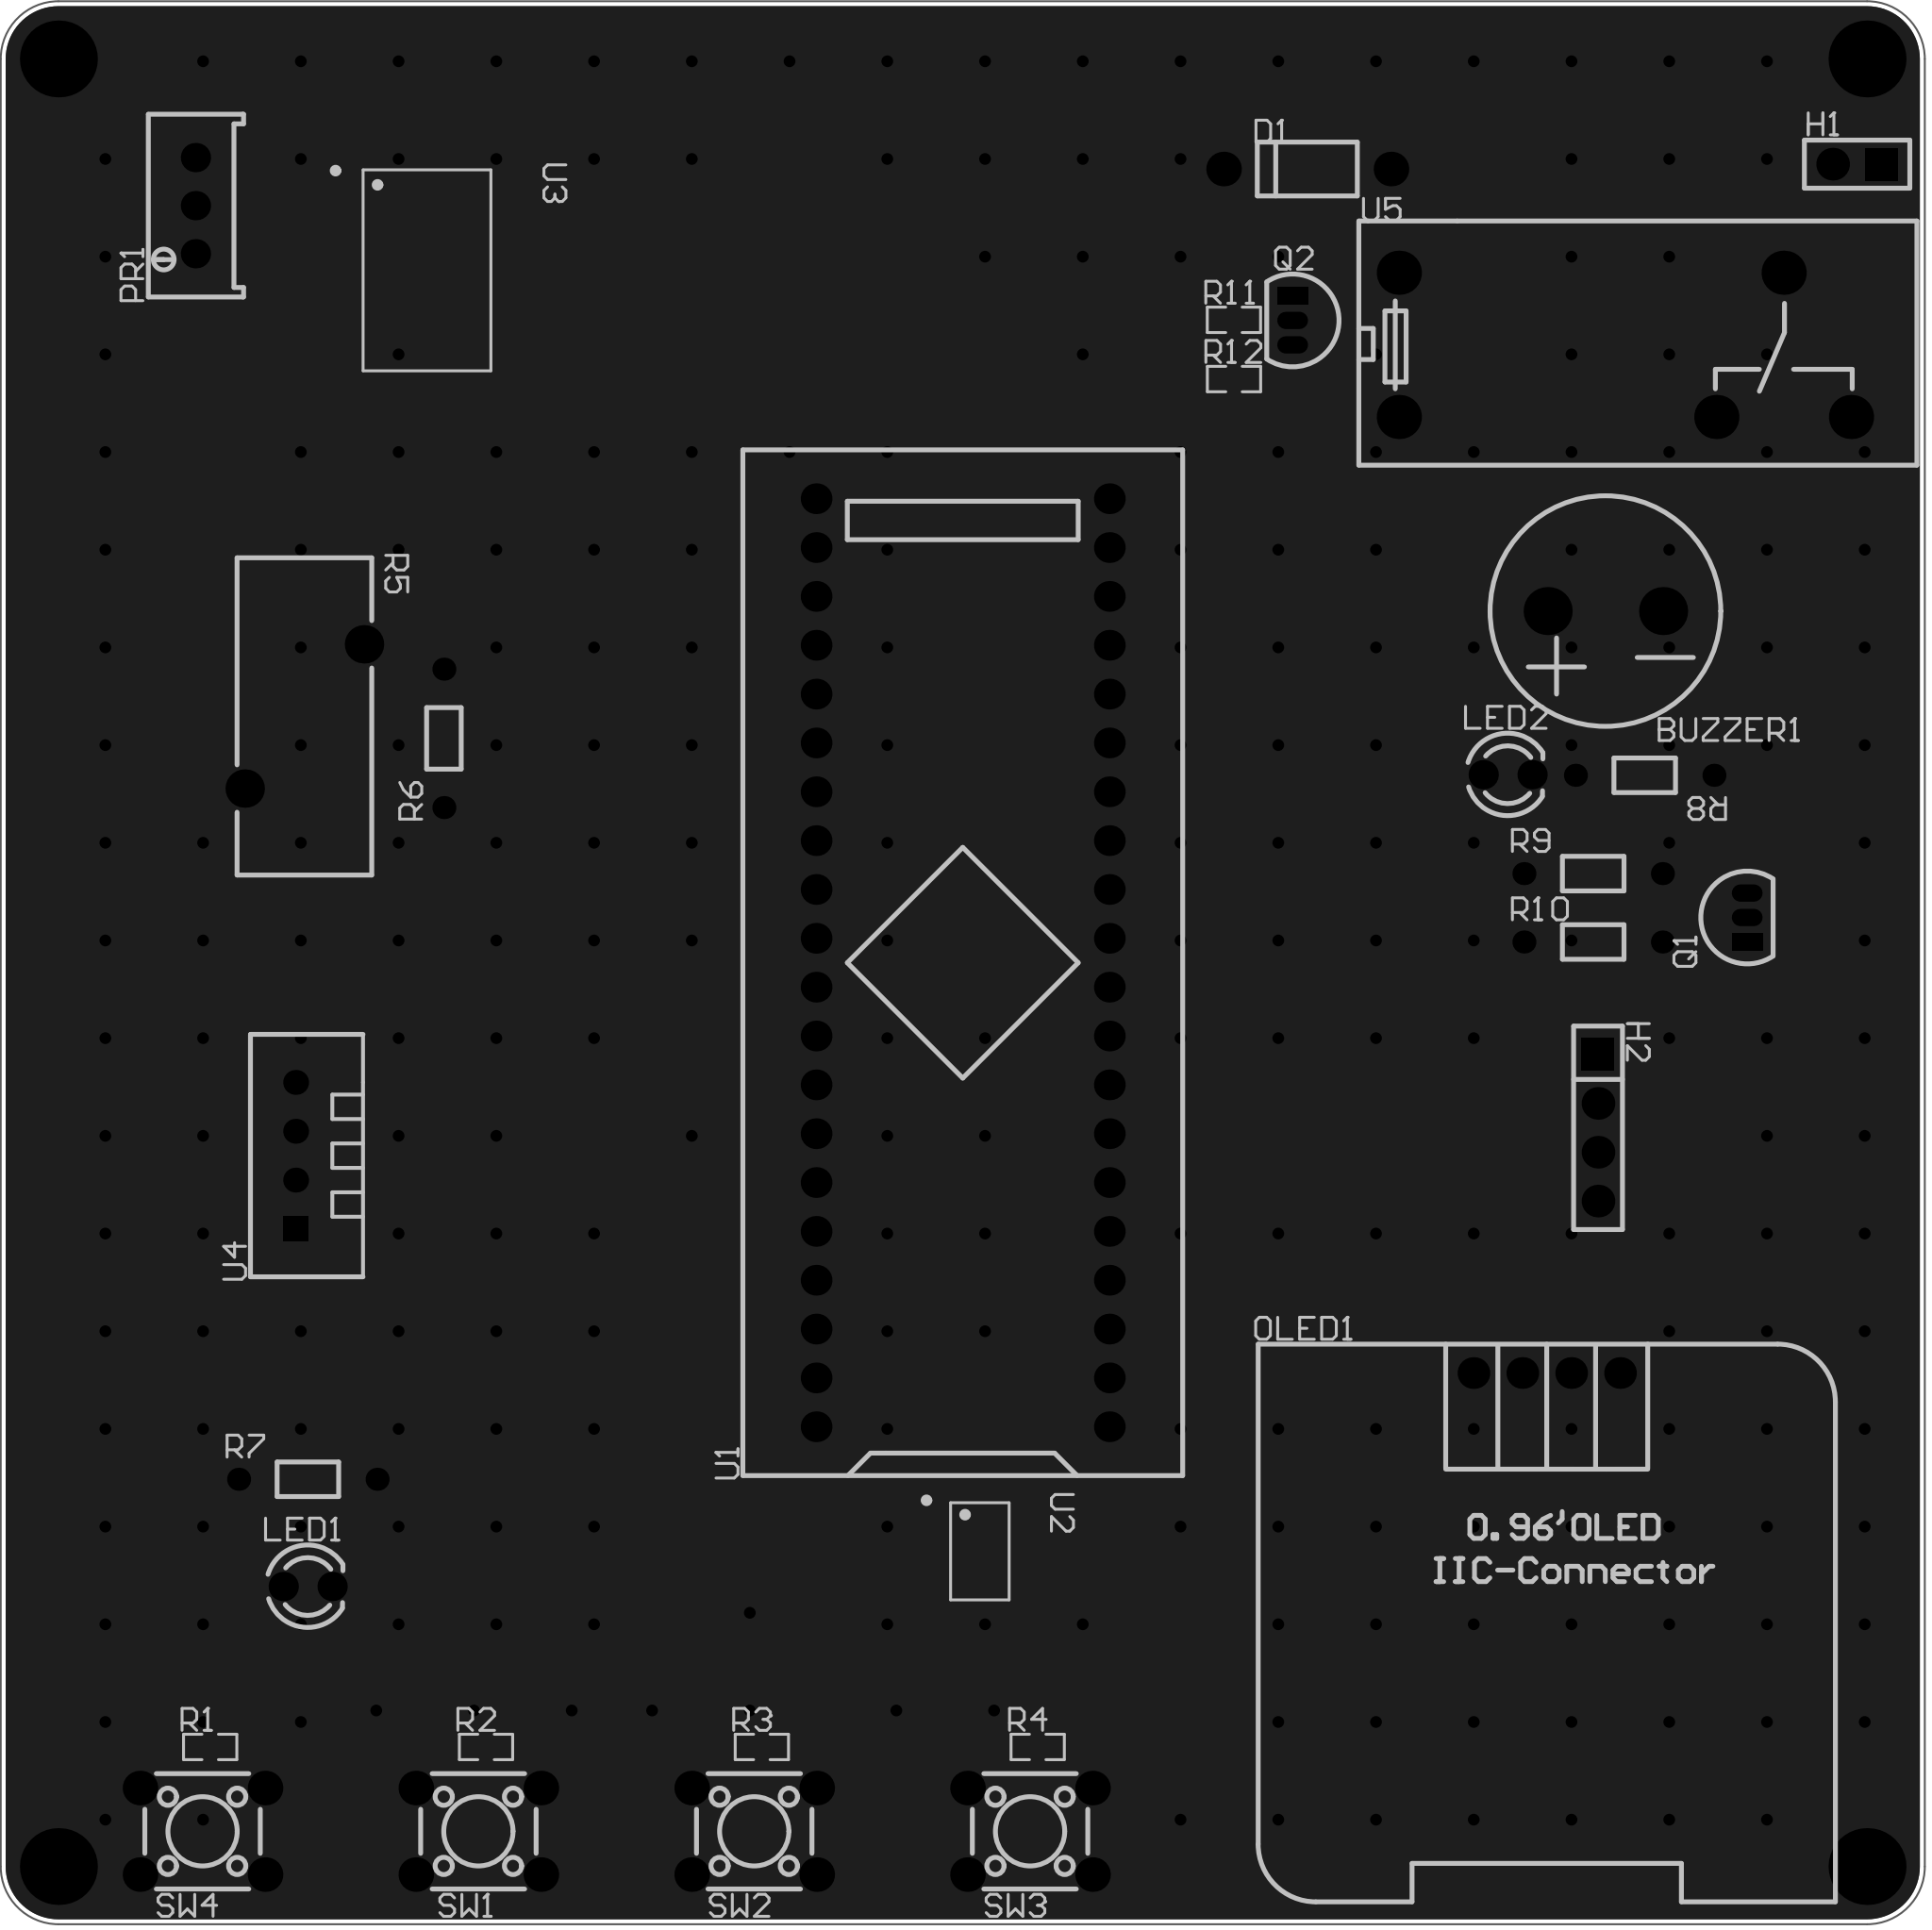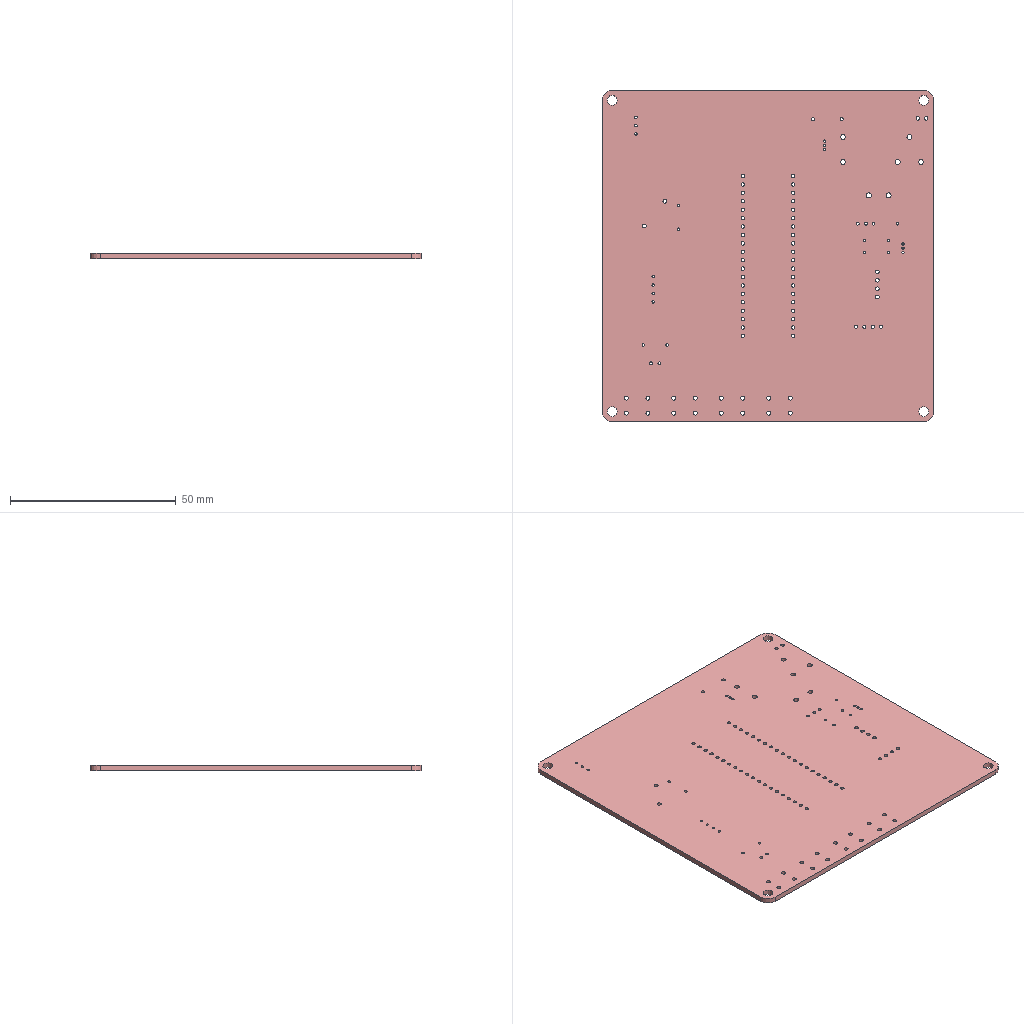Circuit board layout | Altium Designer | box 100 x 100 x 1.6 mm
Layer stack:
# Altium Designer layer stack of  (unit mm; dielectric type: 0 none, 1 core, 2 prepreg, 3 surface material)
index,name,kind,layer,copper_thickness_mm,dielectric_type,dielectric_thickness_mm,dielectric_material,dielectric_constant
0,Top Paste Mask Layer,other,,,,,,
1,Top Silkscreen Layer,other,,,,,,
2,Top Solder Mask Layer,dielectric,,,3,0.01,,3.3
3,Top Layer,copper,Top Layer,0.035,,,,
4,Dielectric1,dielectric,,,3,1.51,FR4,4.5
5,Bottom Layer,copper,Bottom Layer,0.035,,,,
6,Bottom Solder Mask Layer,dielectric,,,3,0.01,,3.3
7,Bottom Silkscreen Layer,other,,,,,,
8,Bottom Paste Mask Layer,other,,,,,,
# drill layer pairs: low layer,high layer
drill_pair,Top Layer,Bottom Layer
Part placement:
Designator,Comment,Layer,Footprint,Center-X(mm),Center-Y(mm),Rotation
BUZZER1,buzzer,TopLayer,BUZ-TH_BD12.0-P6.00-D0.9-RD,174.752,149.225,180
D1,,TopLayer,DO_1N4007,159.258,172.212,0
H1,,TopLayer,HDR-TH_2P-P2.54-V-F,187.833,172.466,180
H2,,TopLayer,HDR-TH_4P-P2.54-V-F,174.368,122.353,270
LED1,,TopLayer,LED_TH-3mm,107.306,98.5,0
LED2,,TopLayer,LED_TH-3mm,169.672,140.716,0
OLED1,,TopLayer,0.96OLED_4P,171.704,109.601,0
PR1,10kΩ,TopLayer,R_3296,101.473,170.307,90
Q1,,TopLayer,S8050_TO_92,182.12,133.291,90
Q2,,TopLayer,S8050_TO_92,158.496,164.338,270
R1,10K,TopLayer,R0603,102.237,90.156,0
R2,10K,TopLayer,R0603,116.573,90.156,0
R3,10K,TopLayer,R0603,130.909,90.156,0
R4,10K,TopLayer,R0603,145.245,90.156,0
R5,3Ω,7A,0.075Ω,TopLayer,RES-TH_L16.5-W7.0-P7.50-D0.8-S6.2,107.134,143.746,270
R6,10kΩ,TopLayer,Res_1/8W,114.385,142.605,90
R7,500Ω,TopLayer,Res_1/8W,107.315,104.076,0
R8,10Ω,TopLayer,Res_1/8W,176.794,140.685,180
R9,1kΩ,TopLayer,Res_1/8W,174.117,135.572,0
R10,10kΩ,TopLayer,Res_1/8W,174.117,132.016,0
R11,1K,TopLayer,R0603,155.444,164.37,0
R12,10K,TopLayer,R0603,155.448,161.29,0
SW1,,TopLayer,SW-TH_4P-L6.0-W6.0-P4.50-LS6.5,116.177,85.769,180
SW2,,TopLayer,SW-TH_4P-L6.0-W6.0-P4.50-LS6.5,130.513,85.769,180
SW3,,TopLayer,SW-TH_4P-L6.0-W6.0-P4.50-LS6.5,144.849,85.769,180
SW4,,TopLayer,SW-TH_4P-L6.0-W6.0-P4.50-LS6.5,101.841,85.769,180
U1,STM32F103C8T6-Card,TopLayer,CONN-TH_L53.3-W22.9_STM32F103C8T6-CARD,141.351,130.937,90
U2,24C02CT-I/SN,TopLayer,SOIC-8_L4.9-W3.9-P1.27-LS6.0-BL,142.24,100.33,270
U3,PCF8591T,TopLayer,SOIC-16_L10.3-W7.5-P1.27-LS10.3-BL,113.505,166.944,270
U4,DHT11,TopLayer,SENSOR-TH_DHT11,106.68,120.904,90
U5,SSKD6132,TopLayer,RELAY-TH_G2R-1,175.768,163.068,0
Pad and via stacks:
# Altium Designer via and pad stacks of  (unit mm). Each distinct definition once, with the count of objects using it.
# via: kind,start_layer,end_layer,hole_mm,diameter_mm,mode(0 simple;1 top-mid-bottom;2 full stack),diameter_per_layer,count,example_net
# pad: kind,layer,hole_mm,hole_type(0 round;1 square;2 slot),plating,top_size,top_shape(1 round;2 rect;3 octagon;9 rounded rect),mid_size,bottom_size,mode,footprint,size_per_layer,count,example
pad,Multi-Layer,3,0,plated,4x4,1,4x4,4x4,0,,,4,1
pad,Multi-Layer,1.5,0,plated,2.5x2.5,1,2.5x2.5,2.5x2.5,0,BUZ-TH_BD12.0-P6.00-D0.9-RD,,2,BUZZER1.1
pad,Multi-Layer,1,0,plated,1.8x1.8,1,1.8x1.8,1.8x1.8,0,DO_1N4007,,2,D1.1
pad,Multi-Layer,1,0,plated,1.7x1.7,2,1.7x1.7,1.7x1.7,0,HDR-TH_2P-P2.54-V-F,,1,H1.1
pad,Multi-Layer,1,0,plated,1.7x1.7,1,1.7x1.7,1.7x1.7,0,HDR-TH_2P-P2.54-V-F,,1,H1.2
pad,Multi-Layer,1.1,0,plated,1.7x1.7,2,1.7x1.7,1.7x1.7,0,HDR-TH_4P-P2.54-V-F,,1,H2.1
pad,Multi-Layer,1.1,0,plated,1.7x1.7,1,1.7x1.7,1.7x1.7,0,HDR-TH_4P-P2.54-V-F,,3,H2.2
pad,Multi-Layer,0.9144,0,plated,1.524x1.524,1,1.524x1.524,1.524x1.524,0,LED_TH-3mm,,4,LED1.1
pad,Multi-Layer,1,0,plated,1.65x1.65,1,1.65x1.65,1.65x1.65,0,0.96OLED_4P,,4,OLED1.4
pad,Multi-Layer,0.762,0,plated,1.524x1.524,1,1.524x1.524,1.524x1.524,0,R_3296,,3,PR1.2
pad,Multi-Layer,0.701,0,plated,0.8992x1.6,2,0.8992x1.6,0.8992x1.6,0,S8050_TO_92,,2,Q1.1
pad,Multi-Layer,0.701,0,plated,0.8992x1.6,1,0.8992x1.6,0.8992x1.6,0,S8050_TO_92,,4,Q1.2
pad,Multi-Layer,1.2,0,plated,2x2,1,2x2,2x2,0,RES-TH_L16.5-W7.0-P7.50-D0.8-S6.2,,2,R5.2
pad,Multi-Layer,0.8001,0,plated,1.199x1.199,1,1.199x1.199,1.199x1.199,0,Res_1/8W,,10,R6.1
pad,Multi-Layer,1.2,0,plated,1.8x1.8,1,1.8x1.8,1.8x1.8,0,SW-TH_4P-L6.0-W6.0-P4.50-LS6.5,,16,SW1.1
pad,Multi-Layer,1,0,plated,1.6x1.6,1,1.6x1.6,1.6x1.6,0,CONN-TH_L53.3-W22.9_STM32F103C8T6-CARD,,40,U1.1
pad,Multi-Layer,0.7112,0,plated,1.295x1.295,2,1.295x1.295,1.295x1.295,0,SENSOR-TH_DHT11,,1,U4.1
pad,Multi-Layer,0.7112,0,plated,1.295x1.295,1,1.295x1.295,1.295x1.295,0,SENSOR-TH_DHT11,,3,U4.2
pad,Multi-Layer,1.5,0,plated,2.3x2.3,1,2.3x2.3,2.3x2.3,0,RELAY-TH_G2R-1,,5,U5.3
pad,Top Layer,0,0,plated,0.8065x0.864,2,0.8065x0.864,0.8065x0.864,0,R0603,,12,R1.2
pad,Top Layer,0,0,plated,0.588x2.045,1,0.588x2.045,0.588x2.045,0,SOIC-8_L4.9-W3.9-P1.27-LS6.0-BL,,8,U2.5
pad,Top Layer,0,0,plated,0.574x2.401,1,0.574x2.401,0.574x2.401,0,SOIC-16_L10.3-W7.5-P1.27-LS10.3-BL,,16,U3.1
via,Top Layer,Bottom Layer,0.3048,0.61,0,,253,GND
Copper pours:
name,layer,net,type(0 solid;1 hatched;2 none)
Bottom Layer-GND,Bottom Layer,GND,0
Top Layer-GND,Top Layer,GND,0